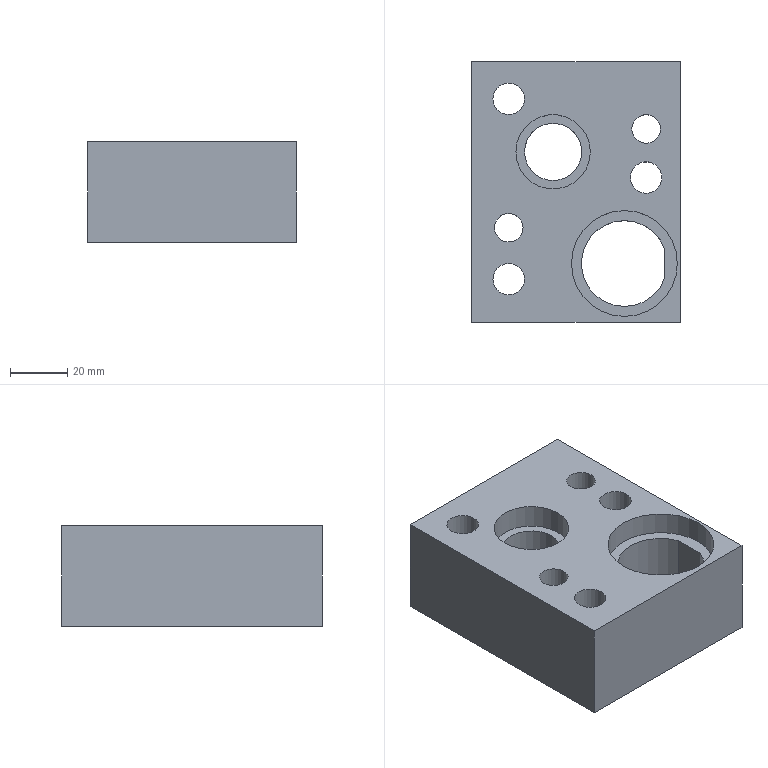Part | NX | features solid 2 | 1 solid | 28 faces | box 73 x 91 x 35 mm | volume 168584 mm3 | plane 14 | cylinder 14 | commonest cylinder face diameters 11 x3 17 x3 10 x2 10.5 x2 20 x1 26 x1
STEP:
#1=CARTESIAN_POINT('',(128.,-184.5,78.));
#2=VERTEX_POINT('',#1);
#3=CARTESIAN_POINT('',(133.5,-184.5,78.));
#4=DIRECTION('',(0.,0.,-1.));
#5=DIRECTION('',(-1.,0.,0.));
#6=AXIS2_PLACEMENT_3D('',#3,#4,#5);
#7=CIRCLE('',#6,5.5);
#8=EDGE_CURVE('',#2,#2,#7,.T.);
#9=ORIENTED_EDGE('',*,*,#8,.T.);
#10=EDGE_LOOP('',(#9));
#11=FACE_BOUND('',#10,.T.);
#12=CARTESIAN_POINT('',(136.,-140.,78.));
#13=VERTEX_POINT('',#12);
#14=CARTESIAN_POINT('',(149.,-140.,78.));
#15=DIRECTION('',(0.,0.,-1.));
#16=DIRECTION('',(-1.,0.,0.));
#17=AXIS2_PLACEMENT_3D('',#14,#15,#16);
#18=CIRCLE('',#17,13.);
#19=EDGE_CURVE('',#13,#13,#18,.F.);
#20=ORIENTED_EDGE('',*,*,#19,.F.);
#21=EDGE_LOOP('',(#20));
#22=FACE_BOUND('',#21,.T.);
#23=CARTESIAN_POINT('',(128.5,-166.5,78.));
#24=VERTEX_POINT('',#23);
#25=CARTESIAN_POINT('',(133.5,-166.5,78.));
#26=DIRECTION('',(0.,0.,-1.));
#27=DIRECTION('',(-1.,0.,0.));
#28=AXIS2_PLACEMENT_3D('',#25,#26,#27);
#29=CIRCLE('',#28,5.);
#30=EDGE_CURVE('',#24,#24,#29,.T.);
#31=ORIENTED_EDGE('',*,*,#30,.T.);
#32=EDGE_LOOP('',(#31));
#33=FACE_BOUND('',#32,.T.);
#34=CARTESIAN_POINT('',(176.,-149.,78.));
#35=VERTEX_POINT('',#34);
#36=CARTESIAN_POINT('',(181.5,-149.,78.));
#37=DIRECTION('',(0.,0.,1.));
#38=DIRECTION('',(-1.,0.,0.));
#39=AXIS2_PLACEMENT_3D('',#36,#37,#38);
#40=CIRCLE('',#39,5.5);
#41=EDGE_CURVE('',#35,#35,#40,.F.);
#42=ORIENTED_EDGE('',*,*,#41,.T.);
#43=EDGE_LOOP('',(#42));
#44=FACE_BOUND('',#43,.T.);
#45=CARTESIAN_POINT('',(176.5,-132.,78.));
#46=VERTEX_POINT('',#45);
#47=CARTESIAN_POINT('',(181.5,-132.,78.));
#48=DIRECTION('',(0.,0.,-1.));
#49=DIRECTION('',(-1.,0.,0.));
#50=AXIS2_PLACEMENT_3D('',#47,#48,#49);
#51=CIRCLE('',#50,5.);
#52=EDGE_CURVE('',#46,#46,#51,.T.);
#53=ORIENTED_EDGE('',*,*,#52,.T.);
#54=EDGE_LOOP('',(#53));
#55=FACE_BOUND('',#54,.T.);
#56=CARTESIAN_POINT('',(139.,-121.5,78.));
#57=VERTEX_POINT('',#56);
#58=CARTESIAN_POINT('',(133.5,-121.5,78.));
#59=DIRECTION('',(0.,0.,1.));
#60=DIRECTION('',(1.,0.,0.));
#61=AXIS2_PLACEMENT_3D('',#58,#59,#60);
#62=CIRCLE('',#61,5.5);
#63=EDGE_CURVE('',#57,#57,#62,.T.);
#64=ORIENTED_EDGE('',*,*,#63,.F.);
#65=EDGE_LOOP('',(#64));
#66=FACE_BOUND('',#65,.T.);
#67=CARTESIAN_POINT('',(193.5,-199.5,78.));
#68=VERTEX_POINT('',#67);
#69=CARTESIAN_POINT('',(193.5,-108.5,78.));
#70=VERTEX_POINT('',#69);
#71=CARTESIAN_POINT('',(193.5,-140.,78.));
#72=DIRECTION('',(0.,-1.,0.));
#73=VECTOR('',#72,1000.);
#74=LINE('',#71,#73);
#75=EDGE_CURVE('',#68,#70,#74,.F.);
#76=ORIENTED_EDGE('',*,*,#75,.T.);
#77=CARTESIAN_POINT('',(120.5,-108.5,78.));
#78=VERTEX_POINT('',#77);
#79=CARTESIAN_POINT('',(149.,-108.5,78.));
#80=DIRECTION('',(1.,0.,0.));
#81=VECTOR('',#80,1000.);
#82=LINE('',#79,#81);
#83=EDGE_CURVE('',#70,#78,#82,.F.);
#84=ORIENTED_EDGE('',*,*,#83,.T.);
#85=CARTESIAN_POINT('',(120.5,-199.5,78.));
#86=VERTEX_POINT('',#85);
#87=CARTESIAN_POINT('',(120.5,-140.,78.));
#88=DIRECTION('',(0.,1.,0.));
#89=VECTOR('',#88,1000.);
#90=LINE('',#87,#89);
#91=EDGE_CURVE('',#78,#86,#90,.F.);
#92=ORIENTED_EDGE('',*,*,#91,.T.);
#93=CARTESIAN_POINT('',(149.,-199.5,78.));
#94=DIRECTION('',(-1.,0.,0.));
#95=VECTOR('',#94,1000.);
#96=LINE('',#93,#95);
#97=EDGE_CURVE('',#86,#68,#96,.F.);
#98=ORIENTED_EDGE('',*,*,#97,.T.);
#99=EDGE_LOOP('',(#76,#84,#92,#98));
#100=FACE_BOUND('',#99,.T.);
#101=CARTESIAN_POINT('',(155.401,-179.,78.));
#102=VERTEX_POINT('',#101);
#103=CARTESIAN_POINT('',(173.901,-179.,78.));
#104=DIRECTION('',(0.,0.,-1.));
#105=DIRECTION('',(-1.,0.,0.));
#106=AXIS2_PLACEMENT_3D('',#103,#104,#105);
#107=CIRCLE('',#106,18.5);
#108=EDGE_CURVE('',#102,#102,#107,.F.);
#109=ORIENTED_EDGE('',*,*,#108,.F.);
#110=EDGE_LOOP('',(#109));
#111=FACE_BOUND('',#110,.T.);
#112=CARTESIAN_POINT('',(149.,-140.,78.));
#113=DIRECTION('',(0.,0.,-1.));
#114=DIRECTION('',(-1.,0.,0.));
#115=AXIS2_PLACEMENT_3D('',#112,#113,#114);
#116=PLANE('',#115);
#117=ADVANCED_FACE('',(#11,#22,#33,#44,#55,#66,#100,#111),#116,.F.);
#118=CARTESIAN_POINT('',(139.,-184.5,63.));
#119=VERTEX_POINT('',#118);
#120=CARTESIAN_POINT('',(133.5,-184.5,63.));
#121=DIRECTION('',(0.,0.,1.));
#122=DIRECTION('',(1.,0.,0.));
#123=AXIS2_PLACEMENT_3D('',#120,#121,#122);
#124=CIRCLE('',#123,5.5);
#125=EDGE_CURVE('',#119,#119,#124,.F.);
#126=ORIENTED_EDGE('',*,*,#125,.F.);
#127=EDGE_LOOP('',(#126));
#128=FACE_BOUND('',#127,.T.);
#129=CARTESIAN_POINT('',(142.,-184.5,63.));
#130=VERTEX_POINT('',#129);
#131=CARTESIAN_POINT('',(133.5,-184.5,63.));
#132=DIRECTION('',(0.,0.,1.));
#133=DIRECTION('',(1.,0.,0.));
#134=AXIS2_PLACEMENT_3D('',#131,#132,#133);
#135=CIRCLE('',#134,8.5);
#136=EDGE_CURVE('',#130,#130,#135,.F.);
#137=ORIENTED_EDGE('',*,*,#136,.T.);
#138=EDGE_LOOP('',(#137));
#139=FACE_BOUND('',#138,.T.);
#140=CARTESIAN_POINT('',(135.874,-185.527,63.));
#141=DIRECTION('',(0.,0.,1.));
#142=DIRECTION('',(1.,0.,0.));
#143=AXIS2_PLACEMENT_3D('',#140,#141,#142);
#144=PLANE('',#143);
#145=ADVANCED_FACE('',(#128,#139),#144,.F.);
#146=ORIENTED_EDGE('',*,*,#136,.F.);
#147=EDGE_LOOP('',(#146));
#148=FACE_BOUND('',#147,.T.);
#149=CARTESIAN_POINT('',(125.,-184.5,43.));
#150=VERTEX_POINT('',#149);
#151=CARTESIAN_POINT('',(133.5,-184.5,43.));
#152=DIRECTION('',(0.,0.,-1.));
#153=DIRECTION('',(-1.,0.,0.));
#154=AXIS2_PLACEMENT_3D('',#151,#152,#153);
#155=CIRCLE('',#154,8.5);
#156=EDGE_CURVE('',#150,#150,#155,.T.);
#157=ORIENTED_EDGE('',*,*,#156,.T.);
#158=EDGE_LOOP('',(#157));
#159=FACE_BOUND('',#158,.T.);
#160=CARTESIAN_POINT('',(133.5,-184.5,43.));
#161=DIRECTION('',(0.,0.,1.));
#162=DIRECTION('',(1.,0.,0.));
#163=AXIS2_PLACEMENT_3D('',#160,#161,#162);
#164=CYLINDRICAL_SURFACE('',#163,8.5);
#165=ADVANCED_FACE('',(#148,#159),#164,.F.);
#166=ORIENTED_EDGE('',*,*,#8,.F.);
#167=EDGE_LOOP('',(#166));
#168=FACE_BOUND('',#167,.T.);
#169=ORIENTED_EDGE('',*,*,#125,.T.);
#170=EDGE_LOOP('',(#169));
#171=FACE_BOUND('',#170,.T.);
#172=CARTESIAN_POINT('',(133.5,-184.5,78.));
#173=DIRECTION('',(0.,0.,1.));
#174=DIRECTION('',(1.,0.,0.));
#175=AXIS2_PLACEMENT_3D('',#172,#173,#174);
#176=CYLINDRICAL_SURFACE('',#175,5.5);
#177=ADVANCED_FACE('',(#168,#171),#176,.F.);
#178=CARTESIAN_POINT('',(139.,-121.5,63.));
#179=VERTEX_POINT('',#178);
#180=CARTESIAN_POINT('',(133.5,-121.5,63.));
#181=DIRECTION('',(0.,0.,1.));
#182=DIRECTION('',(1.,0.,0.));
#183=AXIS2_PLACEMENT_3D('',#180,#181,#182);
#184=CIRCLE('',#183,5.5);
#185=EDGE_CURVE('',#179,#179,#184,.F.);
#186=ORIENTED_EDGE('',*,*,#185,.F.);
#187=EDGE_LOOP('',(#186));
#188=FACE_BOUND('',#187,.T.);
#189=CARTESIAN_POINT('',(142.,-121.5,63.));
#190=VERTEX_POINT('',#189);
#191=CARTESIAN_POINT('',(133.5,-121.5,63.));
#192=DIRECTION('',(0.,0.,1.));
#193=DIRECTION('',(1.,0.,0.));
#194=AXIS2_PLACEMENT_3D('',#191,#192,#193);
#195=CIRCLE('',#194,8.5);
#196=EDGE_CURVE('',#190,#190,#195,.F.);
#197=ORIENTED_EDGE('',*,*,#196,.T.);
#198=EDGE_LOOP('',(#197));
#199=FACE_BOUND('',#198,.T.);
#200=CARTESIAN_POINT('',(135.874,-122.527,63.));
#201=DIRECTION('',(0.,0.,1.));
#202=DIRECTION('',(1.,0.,0.));
#203=AXIS2_PLACEMENT_3D('',#200,#201,#202);
#204=PLANE('',#203);
#205=ADVANCED_FACE('',(#188,#199),#204,.F.);
#206=CARTESIAN_POINT('',(186.5,-132.,58.));
#207=VERTEX_POINT('',#206);
#208=CARTESIAN_POINT('',(181.5,-132.,58.));
#209=DIRECTION('',(0.,0.,1.));
#210=DIRECTION('',(1.,0.,0.));
#211=AXIS2_PLACEMENT_3D('',#208,#209,#210);
#212=CIRCLE('',#211,5.);
#213=EDGE_CURVE('',#207,#207,#212,.F.);
#214=ORIENTED_EDGE('',*,*,#213,.F.);
#215=EDGE_LOOP('',(#214));
#216=FACE_BOUND('',#215,.T.);
#217=CARTESIAN_POINT('',(186.75,-132.,58.));
#218=VERTEX_POINT('',#217);
#219=CARTESIAN_POINT('',(181.5,-132.,58.));
#220=DIRECTION('',(0.,0.,1.));
#221=DIRECTION('',(1.,0.,0.));
#222=AXIS2_PLACEMENT_3D('',#219,#220,#221);
#223=CIRCLE('',#222,5.25);
#224=EDGE_CURVE('',#218,#218,#223,.F.);
#225=ORIENTED_EDGE('',*,*,#224,.T.);
#226=EDGE_LOOP('',(#225));
#227=FACE_BOUND('',#226,.T.);
#228=CARTESIAN_POINT('',(155.126,-122.527,58.));
#229=DIRECTION('',(0.,0.,1.));
#230=DIRECTION('',(-1.,0.,0.));
#231=AXIS2_PLACEMENT_3D('',#228,#229,#230);
#232=PLANE('',#231);
#233=ADVANCED_FACE('',(#216,#227),#232,.F.);
#234=CARTESIAN_POINT('',(176.,-149.,63.));
#235=VERTEX_POINT('',#234);
#236=CARTESIAN_POINT('',(181.5,-149.,63.));
#237=DIRECTION('',(0.,0.,1.));
#238=DIRECTION('',(-1.,0.,0.));
#239=AXIS2_PLACEMENT_3D('',#236,#237,#238);
#240=CIRCLE('',#239,5.5);
#241=EDGE_CURVE('',#235,#235,#240,.F.);
#242=ORIENTED_EDGE('',*,*,#241,.F.);
#243=EDGE_LOOP('',(#242));
#244=FACE_BOUND('',#243,.T.);
#245=CARTESIAN_POINT('',(173.,-149.,63.));
#246=VERTEX_POINT('',#245);
#247=CARTESIAN_POINT('',(181.5,-149.,63.));
#248=DIRECTION('',(0.,0.,1.));
#249=DIRECTION('',(-1.,0.,0.));
#250=AXIS2_PLACEMENT_3D('',#247,#248,#249);
#251=CIRCLE('',#250,8.5);
#252=EDGE_CURVE('',#246,#246,#251,.F.);
#253=ORIENTED_EDGE('',*,*,#252,.T.);
#254=EDGE_LOOP('',(#253));
#255=FACE_BOUND('',#254,.T.);
#256=CARTESIAN_POINT('',(179.126,-147.973,63.));
#257=DIRECTION('',(0.,0.,1.));
#258=DIRECTION('',(-1.,0.,0.));
#259=AXIS2_PLACEMENT_3D('',#256,#257,#258);
#260=PLANE('',#259);
#261=ADVANCED_FACE('',(#244,#255),#260,.F.);
#262=CARTESIAN_POINT('',(138.5,-166.5,58.));
#263=VERTEX_POINT('',#262);
#264=CARTESIAN_POINT('',(133.5,-166.5,58.));
#265=DIRECTION('',(0.,0.,1.));
#266=DIRECTION('',(1.,0.,0.));
#267=AXIS2_PLACEMENT_3D('',#264,#265,#266);
#268=CIRCLE('',#267,5.);
#269=EDGE_CURVE('',#263,#263,#268,.F.);
#270=ORIENTED_EDGE('',*,*,#269,.F.);
#271=EDGE_LOOP('',(#270));
#272=FACE_BOUND('',#271,.T.);
#273=CARTESIAN_POINT('',(138.75,-166.5,58.));
#274=VERTEX_POINT('',#273);
#275=CARTESIAN_POINT('',(133.5,-166.5,58.));
#276=DIRECTION('',(0.,0.,1.));
#277=DIRECTION('',(1.,0.,0.));
#278=AXIS2_PLACEMENT_3D('',#275,#276,#277);
#279=CIRCLE('',#278,5.25);
#280=EDGE_CURVE('',#274,#274,#279,.F.);
#281=ORIENTED_EDGE('',*,*,#280,.T.);
#282=EDGE_LOOP('',(#281));
#283=FACE_BOUND('',#282,.T.);
#284=CARTESIAN_POINT('',(155.126,-116.527,58.));
#285=DIRECTION('',(0.,0.,1.));
#286=DIRECTION('',(-1.,0.,0.));
#287=AXIS2_PLACEMENT_3D('',#284,#285,#286);
#288=PLANE('',#287);
#289=ADVANCED_FACE('',(#272,#283),#288,.F.);
#290=CARTESIAN_POINT('',(159.,-140.,69.7));
#291=VERTEX_POINT('',#290);
#292=CARTESIAN_POINT('',(149.,-140.,69.7));
#293=DIRECTION('',(0.,0.,1.));
#294=DIRECTION('',(1.,0.,0.));
#295=AXIS2_PLACEMENT_3D('',#292,#293,#294);
#296=CIRCLE('',#295,10.);
#297=EDGE_CURVE('',#291,#291,#296,.F.);
#298=ORIENTED_EDGE('',*,*,#297,.T.);
#299=EDGE_LOOP('',(#298));
#300=FACE_BOUND('',#299,.T.);
#301=CARTESIAN_POINT('',(162.,-140.,69.7));
#302=VERTEX_POINT('',#301);
#303=CARTESIAN_POINT('',(149.,-140.,69.7));
#304=DIRECTION('',(0.,0.,1.));
#305=DIRECTION('',(1.,0.,0.));
#306=AXIS2_PLACEMENT_3D('',#303,#304,#305);
#307=CIRCLE('',#306,13.);
#308=EDGE_CURVE('',#302,#302,#307,.F.);
#309=ORIENTED_EDGE('',*,*,#308,.F.);
#310=EDGE_LOOP('',(#309));
#311=FACE_BOUND('',#310,.T.);
#312=CARTESIAN_POINT('',(149.,-140.,69.7));
#313=DIRECTION('',(0.,0.,1.));
#314=DIRECTION('',(1.,0.,0.));
#315=AXIS2_PLACEMENT_3D('',#312,#313,#314);
#316=PLANE('',#315);
#317=ADVANCED_FACE('',(#300,#311),#316,.T.);
#318=ORIENTED_EDGE('',*,*,#97,.F.);
#319=CARTESIAN_POINT('',(120.5,-199.5,43.));
#320=VERTEX_POINT('',#319);
#321=CARTESIAN_POINT('',(120.5,-199.5,78.));
#322=DIRECTION('',(0.,0.,-1.));
#323=VECTOR('',#322,1000.);
#324=LINE('',#321,#323);
#325=EDGE_CURVE('',#86,#320,#324,.T.);
#326=ORIENTED_EDGE('',*,*,#325,.T.);
#327=CARTESIAN_POINT('',(193.5,-199.5,43.));
#328=VERTEX_POINT('',#327);
#329=CARTESIAN_POINT('',(149.,-199.5,43.));
#330=DIRECTION('',(-1.,0.,0.));
#331=VECTOR('',#330,1000.);
#332=LINE('',#329,#331);
#333=EDGE_CURVE('',#320,#328,#332,.F.);
#334=ORIENTED_EDGE('',*,*,#333,.T.);
#335=CARTESIAN_POINT('',(193.5,-199.5,78.));
#336=DIRECTION('',(0.,0.,-1.));
#337=VECTOR('',#336,1000.);
#338=LINE('',#335,#337);
#339=EDGE_CURVE('',#68,#328,#338,.T.);
#340=ORIENTED_EDGE('',*,*,#339,.F.);
#341=EDGE_LOOP('',(#318,#326,#334,#340));
#342=FACE_BOUND('',#341,.T.);
#343=CARTESIAN_POINT('',(149.,-199.5,78.));
#344=DIRECTION('',(0.,1.,0.));
#345=DIRECTION('',(1.,0.,0.));
#346=AXIS2_PLACEMENT_3D('',#343,#344,#345);
#347=PLANE('',#346);
#348=ADVANCED_FACE('',(#342),#347,.F.);
#349=ORIENTED_EDGE('',*,*,#325,.F.);
#350=ORIENTED_EDGE('',*,*,#91,.F.);
#351=CARTESIAN_POINT('',(120.5,-108.5,43.));
#352=VERTEX_POINT('',#351);
#353=CARTESIAN_POINT('',(120.5,-108.5,78.));
#354=DIRECTION('',(0.,0.,-1.));
#355=VECTOR('',#354,1000.);
#356=LINE('',#353,#355);
#357=EDGE_CURVE('',#78,#352,#356,.T.);
#358=ORIENTED_EDGE('',*,*,#357,.T.);
#359=CARTESIAN_POINT('',(120.5,-140.,43.));
#360=DIRECTION('',(0.,1.,0.));
#361=VECTOR('',#360,1000.);
#362=LINE('',#359,#361);
#363=EDGE_CURVE('',#352,#320,#362,.F.);
#364=ORIENTED_EDGE('',*,*,#363,.T.);
#365=EDGE_LOOP('',(#349,#350,#358,#364));
#366=FACE_BOUND('',#365,.T.);
#367=CARTESIAN_POINT('',(120.5,-140.,78.));
#368=DIRECTION('',(1.,0.,0.));
#369=DIRECTION('',(0.,-1.,0.));
#370=AXIS2_PLACEMENT_3D('',#367,#368,#369);
#371=PLANE('',#370);
#372=ADVANCED_FACE('',(#366),#371,.F.);
#373=ORIENTED_EDGE('',*,*,#357,.F.);
#374=ORIENTED_EDGE('',*,*,#83,.F.);
#375=CARTESIAN_POINT('',(193.5,-108.5,43.));
#376=VERTEX_POINT('',#375);
#377=CARTESIAN_POINT('',(193.5,-108.5,78.));
#378=DIRECTION('',(0.,0.,-1.));
#379=VECTOR('',#378,1000.);
#380=LINE('',#377,#379);
#381=EDGE_CURVE('',#70,#376,#380,.T.);
#382=ORIENTED_EDGE('',*,*,#381,.T.);
#383=CARTESIAN_POINT('',(149.,-108.5,43.));
#384=DIRECTION('',(1.,0.,0.));
#385=VECTOR('',#384,1000.);
#386=LINE('',#383,#385);
#387=EDGE_CURVE('',#376,#352,#386,.F.);
#388=ORIENTED_EDGE('',*,*,#387,.T.);
#389=EDGE_LOOP('',(#373,#374,#382,#388));
#390=FACE_BOUND('',#389,.T.);
#391=CARTESIAN_POINT('',(149.,-108.5,78.));
#392=DIRECTION('',(0.,-1.,0.));
#393=DIRECTION('',(-1.,0.,0.));
#394=AXIS2_PLACEMENT_3D('',#391,#392,#393);
#395=PLANE('',#394);
#396=ADVANCED_FACE('',(#390),#395,.F.);
#397=ORIENTED_EDGE('',*,*,#381,.F.);
#398=ORIENTED_EDGE('',*,*,#75,.F.);
#399=ORIENTED_EDGE('',*,*,#339,.T.);
#400=CARTESIAN_POINT('',(193.5,-140.,43.));
#401=DIRECTION('',(0.,-1.,0.));
#402=VECTOR('',#401,1000.);
#403=LINE('',#400,#402);
#404=EDGE_CURVE('',#328,#376,#403,.F.);
#405=ORIENTED_EDGE('',*,*,#404,.T.);
#406=EDGE_LOOP('',(#397,#398,#399,#405));
#407=FACE_BOUND('',#406,.T.);
#408=CARTESIAN_POINT('',(193.5,-140.,78.));
#409=DIRECTION('',(-1.,0.,0.));
#410=DIRECTION('',(0.,1.,0.));
#411=AXIS2_PLACEMENT_3D('',#408,#409,#410);
#412=PLANE('',#411);
#413=ADVANCED_FACE('',(#407),#412,.F.);
#414=ORIENTED_EDGE('',*,*,#63,.T.);
#415=EDGE_LOOP('',(#414));
#416=FACE_BOUND('',#415,.T.);
#417=ORIENTED_EDGE('',*,*,#185,.T.);
#418=EDGE_LOOP('',(#417));
#419=FACE_BOUND('',#418,.T.);
#420=CARTESIAN_POINT('',(133.5,-121.5,78.));
#421=DIRECTION('',(0.,0.,1.));
#422=DIRECTION('',(1.,0.,0.));
#423=AXIS2_PLACEMENT_3D('',#420,#421,#422);
#424=CYLINDRICAL_SURFACE('',#423,5.5);
#425=ADVANCED_FACE('',(#416,#419),#424,.F.);
#426=ORIENTED_EDGE('',*,*,#52,.F.);
#427=EDGE_LOOP('',(#426));
#428=FACE_BOUND('',#427,.T.);
#429=ORIENTED_EDGE('',*,*,#213,.T.);
#430=EDGE_LOOP('',(#429));
#431=FACE_BOUND('',#430,.T.);
#432=CARTESIAN_POINT('',(181.5,-132.,78.));
#433=DIRECTION('',(0.,0.,1.));
#434=DIRECTION('',(-1.,0.,0.));
#435=AXIS2_PLACEMENT_3D('',#432,#433,#434);
#436=CYLINDRICAL_SURFACE('',#435,5.);
#437=ADVANCED_FACE('',(#428,#431),#436,.F.);
#438=ORIENTED_EDGE('',*,*,#41,.F.);
#439=EDGE_LOOP('',(#438));
#440=FACE_BOUND('',#439,.T.);
#441=ORIENTED_EDGE('',*,*,#241,.T.);
#442=EDGE_LOOP('',(#441));
#443=FACE_BOUND('',#442,.T.);
#444=CARTESIAN_POINT('',(181.5,-149.,78.));
#445=DIRECTION('',(0.,0.,1.));
#446=DIRECTION('',(-1.,0.,0.));
#447=AXIS2_PLACEMENT_3D('',#444,#445,#446);
#448=CYLINDRICAL_SURFACE('',#447,5.5);
#449=ADVANCED_FACE('',(#440,#443),#448,.F.);
#450=ORIENTED_EDGE('',*,*,#30,.F.);
#451=EDGE_LOOP('',(#450));
#452=FACE_BOUND('',#451,.T.);
#453=ORIENTED_EDGE('',*,*,#269,.T.);
#454=EDGE_LOOP('',(#453));
#455=FACE_BOUND('',#454,.T.);
#456=CARTESIAN_POINT('',(133.5,-166.5,78.));
#457=DIRECTION('',(0.,0.,1.));
#458=DIRECTION('',(1.,0.,0.));
#459=AXIS2_PLACEMENT_3D('',#456,#457,#458);
#460=CYLINDRICAL_SURFACE('',#459,5.);
#461=ADVANCED_FACE('',(#452,#455),#460,.F.);
#462=ORIENTED_EDGE('',*,*,#19,.T.);
#463=EDGE_LOOP('',(#462));
#464=FACE_BOUND('',#463,.T.);
#465=ORIENTED_EDGE('',*,*,#308,.T.);
#466=EDGE_LOOP('',(#465));
#467=FACE_BOUND('',#466,.T.);
#468=CARTESIAN_POINT('',(149.,-140.,82.));
#469=DIRECTION('',(0.,0.,-1.));
#470=DIRECTION('',(-1.,0.,0.));
#471=AXIS2_PLACEMENT_3D('',#468,#469,#470);
#472=CYLINDRICAL_SURFACE('',#471,13.);
#473=ADVANCED_FACE('',(#464,#467),#472,.F.);
#474=ORIENTED_EDGE('',*,*,#196,.F.);
#475=EDGE_LOOP('',(#474));
#476=FACE_BOUND('',#475,.T.);
#477=CARTESIAN_POINT('',(142.,-121.5,43.));
#478=VERTEX_POINT('',#477);
#479=CARTESIAN_POINT('',(133.5,-121.5,43.));
#480=DIRECTION('',(0.,0.,1.));
#481=DIRECTION('',(1.,0.,0.));
#482=AXIS2_PLACEMENT_3D('',#479,#480,#481);
#483=CIRCLE('',#482,8.5);
#484=EDGE_CURVE('',#478,#478,#483,.T.);
#485=ORIENTED_EDGE('',*,*,#484,.F.);
#486=EDGE_LOOP('',(#485));
#487=FACE_BOUND('',#486,.T.);
#488=CARTESIAN_POINT('',(133.5,-121.5,43.));
#489=DIRECTION('',(0.,0.,1.));
#490=DIRECTION('',(1.,0.,0.));
#491=AXIS2_PLACEMENT_3D('',#488,#489,#490);
#492=CYLINDRICAL_SURFACE('',#491,8.5);
#493=ADVANCED_FACE('',(#476,#487),#492,.F.);
#494=ORIENTED_EDGE('',*,*,#224,.F.);
#495=EDGE_LOOP('',(#494));
#496=FACE_BOUND('',#495,.T.);
#497=CARTESIAN_POINT('',(176.25,-132.,43.));
#498=VERTEX_POINT('',#497);
#499=CARTESIAN_POINT('',(181.5,-132.,43.));
#500=DIRECTION('',(0.,0.,-1.));
#501=DIRECTION('',(-1.,0.,0.));
#502=AXIS2_PLACEMENT_3D('',#499,#500,#501);
#503=CIRCLE('',#502,5.25);
#504=EDGE_CURVE('',#498,#498,#503,.F.);
#505=ORIENTED_EDGE('',*,*,#504,.F.);
#506=EDGE_LOOP('',(#505));
#507=FACE_BOUND('',#506,.T.);
#508=CARTESIAN_POINT('',(181.5,-132.,43.));
#509=DIRECTION('',(0.,0.,1.));
#510=DIRECTION('',(-1.,0.,0.));
#511=AXIS2_PLACEMENT_3D('',#508,#509,#510);
#512=CYLINDRICAL_SURFACE('',#511,5.25);
#513=ADVANCED_FACE('',(#496,#507),#512,.F.);
#514=ORIENTED_EDGE('',*,*,#252,.F.);
#515=EDGE_LOOP('',(#514));
#516=FACE_BOUND('',#515,.T.);
#517=CARTESIAN_POINT('',(173.,-149.,43.));
#518=VERTEX_POINT('',#517);
#519=CARTESIAN_POINT('',(181.5,-149.,43.));
#520=DIRECTION('',(0.,0.,1.));
#521=DIRECTION('',(-1.,0.,0.));
#522=AXIS2_PLACEMENT_3D('',#519,#520,#521);
#523=CIRCLE('',#522,8.5);
#524=EDGE_CURVE('',#518,#518,#523,.T.);
#525=ORIENTED_EDGE('',*,*,#524,.F.);
#526=EDGE_LOOP('',(#525));
#527=FACE_BOUND('',#526,.T.);
#528=CARTESIAN_POINT('',(181.5,-149.,43.));
#529=DIRECTION('',(0.,0.,1.));
#530=DIRECTION('',(-1.,0.,0.));
#531=AXIS2_PLACEMENT_3D('',#528,#529,#530);
#532=CYLINDRICAL_SURFACE('',#531,8.5);
#533=ADVANCED_FACE('',(#516,#527),#532,.F.);
#534=ORIENTED_EDGE('',*,*,#280,.F.);
#535=EDGE_LOOP('',(#534));
#536=FACE_BOUND('',#535,.T.);
#537=CARTESIAN_POINT('',(128.25,-166.5,43.));
#538=VERTEX_POINT('',#537);
#539=CARTESIAN_POINT('',(133.5,-166.5,43.));
#540=DIRECTION('',(0.,0.,-1.));
#541=DIRECTION('',(-1.,0.,0.));
#542=AXIS2_PLACEMENT_3D('',#539,#540,#541);
#543=CIRCLE('',#542,5.25);
#544=EDGE_CURVE('',#538,#538,#543,.F.);
#545=ORIENTED_EDGE('',*,*,#544,.F.);
#546=EDGE_LOOP('',(#545));
#547=FACE_BOUND('',#546,.T.);
#548=CARTESIAN_POINT('',(133.5,-166.5,43.));
#549=DIRECTION('',(0.,0.,1.));
#550=DIRECTION('',(1.,0.,0.));
#551=AXIS2_PLACEMENT_3D('',#548,#549,#550);
#552=CYLINDRICAL_SURFACE('',#551,5.25);
#553=ADVANCED_FACE('',(#536,#547),#552,.F.);
#554=CARTESIAN_POINT('',(139.,-140.,43.));
#555=VERTEX_POINT('',#554);
#556=CARTESIAN_POINT('',(149.,-140.,43.));
#557=DIRECTION('',(0.,0.,-1.));
#558=DIRECTION('',(-1.,0.,0.));
#559=AXIS2_PLACEMENT_3D('',#556,#557,#558);
#560=CIRCLE('',#559,10.);
#561=EDGE_CURVE('',#555,#555,#560,.F.);
#562=ORIENTED_EDGE('',*,*,#561,.F.);
#563=EDGE_LOOP('',(#562));
#564=FACE_BOUND('',#563,.T.);
#565=ORIENTED_EDGE('',*,*,#297,.F.);
#566=EDGE_LOOP('',(#565));
#567=FACE_BOUND('',#566,.T.);
#568=CARTESIAN_POINT('',(149.,-140.,82.));
#569=DIRECTION('',(0.,0.,-1.));
#570=DIRECTION('',(-1.,0.,0.));
#571=AXIS2_PLACEMENT_3D('',#568,#569,#570);
#572=CYLINDRICAL_SURFACE('',#571,10.);
#573=ADVANCED_FACE('',(#564,#567),#572,.F.);
#574=CARTESIAN_POINT('',(187.901,-184.385,43.));
#575=VERTEX_POINT('',#574);
#576=CARTESIAN_POINT('',(187.901,-173.615,43.));
#577=VERTEX_POINT('',#576);
#578=CARTESIAN_POINT('',(173.901,-179.,43.));
#579=DIRECTION('',(0.,0.,-1.));
#580=DIRECTION('',(-1.,0.,0.));
#581=AXIS2_PLACEMENT_3D('',#578,#579,#580);
#582=CIRCLE('',#581,15.);
#583=EDGE_CURVE('',#575,#577,#582,.T.);
#584=ORIENTED_EDGE('',*,*,#583,.F.);
#585=CARTESIAN_POINT('',(187.901,-140.,43.));
#586=DIRECTION('',(0.,1.,0.));
#587=VECTOR('',#586,1000.);
#588=LINE('',#585,#587);
#589=EDGE_CURVE('',#575,#577,#588,.T.);
#590=ORIENTED_EDGE('',*,*,#589,.T.);
#591=EDGE_LOOP('',(#584,#590));
#592=FACE_BOUND('',#591,.T.);
#593=ORIENTED_EDGE('',*,*,#156,.F.);
#594=EDGE_LOOP('',(#593));
#595=FACE_BOUND('',#594,.T.);
#596=ORIENTED_EDGE('',*,*,#561,.T.);
#597=EDGE_LOOP('',(#596));
#598=FACE_BOUND('',#597,.T.);
#599=ORIENTED_EDGE('',*,*,#544,.T.);
#600=EDGE_LOOP('',(#599));
#601=FACE_BOUND('',#600,.T.);
#602=ORIENTED_EDGE('',*,*,#524,.T.);
#603=EDGE_LOOP('',(#602));
#604=FACE_BOUND('',#603,.T.);
#605=ORIENTED_EDGE('',*,*,#504,.T.);
#606=EDGE_LOOP('',(#605));
#607=FACE_BOUND('',#606,.T.);
#608=ORIENTED_EDGE('',*,*,#484,.T.);
#609=EDGE_LOOP('',(#608));
#610=FACE_BOUND('',#609,.T.);
#611=ORIENTED_EDGE('',*,*,#404,.F.);
#612=ORIENTED_EDGE('',*,*,#333,.F.);
#613=ORIENTED_EDGE('',*,*,#363,.F.);
#614=ORIENTED_EDGE('',*,*,#387,.F.);
#615=EDGE_LOOP('',(#611,#612,#613,#614));
#616=FACE_BOUND('',#615,.T.);
#617=CARTESIAN_POINT('',(149.,-140.,43.));
#618=DIRECTION('',(0.,0.,-1.));
#619=DIRECTION('',(-1.,0.,0.));
#620=AXIS2_PLACEMENT_3D('',#617,#618,#619);
#621=PLANE('',#620);
#622=ADVANCED_FACE('',(#592,#595,#598,#601,#604,#607,#610,#616),#621,.T.);
#623=ORIENTED_EDGE('',*,*,#583,.T.);
#624=CARTESIAN_POINT('',(187.901,-173.615,70.));
#625=VERTEX_POINT('',#624);
#626=CARTESIAN_POINT('',(187.901,-173.615,-33.));
#627=DIRECTION('',(0.,0.,1.));
#628=VECTOR('',#627,1000.);
#629=LINE('',#626,#628);
#630=EDGE_CURVE('',#577,#625,#629,.T.);
#631=ORIENTED_EDGE('',*,*,#630,.T.);
#632=CARTESIAN_POINT('',(187.901,-184.385,70.));
#633=VERTEX_POINT('',#632);
#634=CARTESIAN_POINT('',(173.901,-179.,70.));
#635=DIRECTION('',(0.,0.,1.));
#636=DIRECTION('',(1.,0.,0.));
#637=AXIS2_PLACEMENT_3D('',#634,#635,#636);
#638=CIRCLE('',#637,15.);
#639=EDGE_CURVE('',#625,#633,#638,.T.);
#640=ORIENTED_EDGE('',*,*,#639,.T.);
#641=CARTESIAN_POINT('',(187.901,-184.385,-33.));
#642=DIRECTION('',(0.,0.,1.));
#643=VECTOR('',#642,1000.);
#644=LINE('',#641,#643);
#645=EDGE_CURVE('',#633,#575,#644,.F.);
#646=ORIENTED_EDGE('',*,*,#645,.T.);
#647=EDGE_LOOP('',(#623,#631,#640,#646));
#648=FACE_BOUND('',#647,.T.);
#649=CARTESIAN_POINT('',(173.901,-179.,-33.));
#650=DIRECTION('',(0.,0.,1.));
#651=DIRECTION('',(1.,0.,0.));
#652=AXIS2_PLACEMENT_3D('',#649,#650,#651);
#653=CYLINDRICAL_SURFACE('',#652,15.);
#654=ADVANCED_FACE('',(#648),#653,.F.);
#655=ORIENTED_EDGE('',*,*,#639,.F.);
#656=CARTESIAN_POINT('',(187.901,-145.,70.));
#657=DIRECTION('',(0.,1.,0.));
#658=VECTOR('',#657,1000.);
#659=LINE('',#656,#658);
#660=EDGE_CURVE('',#633,#625,#659,.T.);
#661=ORIENTED_EDGE('',*,*,#660,.F.);
#662=EDGE_LOOP('',(#655,#661));
#663=FACE_BOUND('',#662,.T.);
#664=CARTESIAN_POINT('',(192.401,-179.,70.));
#665=VERTEX_POINT('',#664);
#666=CARTESIAN_POINT('',(173.901,-179.,70.));
#667=DIRECTION('',(0.,0.,1.));
#668=DIRECTION('',(1.,0.,0.));
#669=AXIS2_PLACEMENT_3D('',#666,#667,#668);
#670=CIRCLE('',#669,18.5);
#671=EDGE_CURVE('',#665,#665,#670,.F.);
#672=ORIENTED_EDGE('',*,*,#671,.F.);
#673=EDGE_LOOP('',(#672));
#674=FACE_BOUND('',#673,.T.);
#675=CARTESIAN_POINT('',(173.901,-179.,70.));
#676=DIRECTION('',(0.,0.,1.));
#677=DIRECTION('',(1.,0.,0.));
#678=AXIS2_PLACEMENT_3D('',#675,#676,#677);
#679=PLANE('',#678);
#680=ADVANCED_FACE('',(#663,#674),#679,.T.);
#681=ORIENTED_EDGE('',*,*,#660,.T.);
#682=ORIENTED_EDGE('',*,*,#630,.F.);
#683=ORIENTED_EDGE('',*,*,#589,.F.);
#684=ORIENTED_EDGE('',*,*,#645,.F.);
#685=EDGE_LOOP('',(#681,#682,#683,#684));
#686=FACE_BOUND('',#685,.T.);
#687=CARTESIAN_POINT('',(187.901,-145.,70.));
#688=DIRECTION('',(-1.,0.,0.));
#689=DIRECTION('',(0.,0.,1.));
#690=AXIS2_PLACEMENT_3D('',#687,#688,#689);
#691=PLANE('',#690);
#692=ADVANCED_FACE('',(#686),#691,.T.);
#693=ORIENTED_EDGE('',*,*,#671,.T.);
#694=EDGE_LOOP('',(#693));
#695=FACE_BOUND('',#694,.T.);
#696=ORIENTED_EDGE('',*,*,#108,.T.);
#697=EDGE_LOOP('',(#696));
#698=FACE_BOUND('',#697,.T.);
#699=CARTESIAN_POINT('',(173.901,-179.,87.));
#700=DIRECTION('',(0.,0.,1.));
#701=DIRECTION('',(1.,0.,0.));
#702=AXIS2_PLACEMENT_3D('',#699,#700,#701);
#703=CYLINDRICAL_SURFACE('',#702,18.5);
#704=ADVANCED_FACE('',(#695,#698),#703,.F.);
#705=CLOSED_SHELL('',(#117,#145,#165,#177,#205,#233,#261,#289,#317,#348,#372,#396,#413,#425,#437,#449,#461,#473,#493,#513,#533,#553,#573,#622,#654,#680,#692,#704));
#706=MANIFOLD_SOLID_BREP('',#705);
#707=(LENGTH_UNIT()NAMED_UNIT(*)SI_UNIT(.MILLI.,.METRE.));
#708=UNCERTAINTY_MEASURE_WITH_UNIT(LENGTH_MEASURE(0.00001),#707,'','');
#709=(NAMED_UNIT(*)PLANE_ANGLE_UNIT()SI_UNIT($,.RADIAN.));
#710=(NAMED_UNIT(*)SI_UNIT($,.STERADIAN.)SOLID_ANGLE_UNIT());
#711=(GEOMETRIC_REPRESENTATION_CONTEXT(3)GLOBAL_UNCERTAINTY_ASSIGNED_CONTEXT((#708))GLOBAL_UNIT_ASSIGNED_CONTEXT((#707,#709,#710))REPRESENTATION_CONTEXT('',''));
#712=ADVANCED_BREP_SHAPE_REPRESENTATION('',(#706),#711);